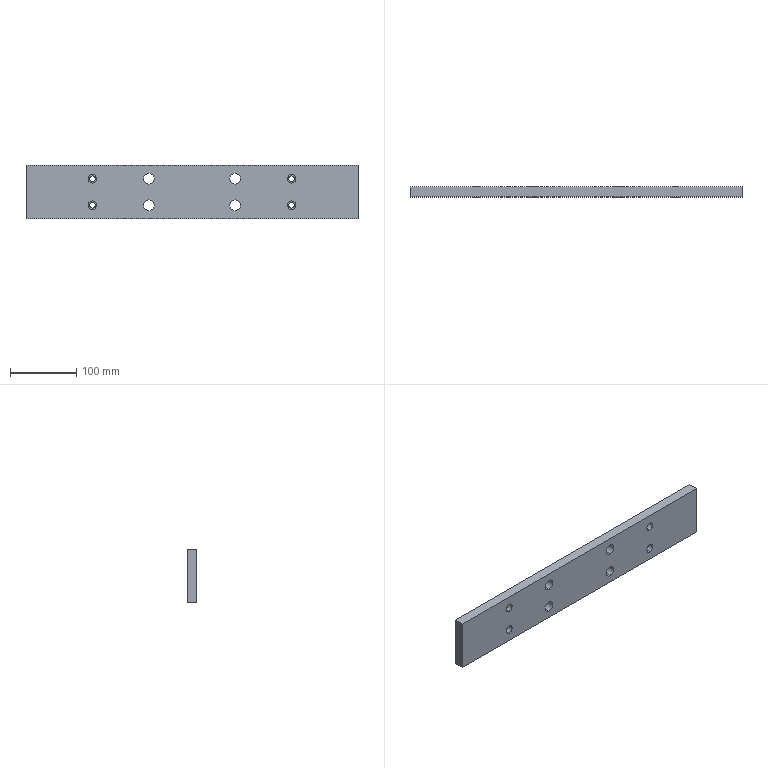Part | SolidWorks | features BaseBody 1 | 1 solid | 34 faces | box 500 x 15 x 80 mm | volume 581983 mm3 | cylinder 24 | plane 10 | commonest cylinder face diameters 8.4 x8 13 x8 16 x8
STEP:
#1=CARTESIAN_POINT('',(150.,92.,158.921));
#2=VERTEX_POINT('',#1);
#3=CARTESIAN_POINT('',(150.,92.,167.321));
#4=VERTEX_POINT('',#3);
#5=CARTESIAN_POINT('',(150.,92.,163.121));
#6=DIRECTION('',(0.,1.,0.));
#7=DIRECTION('',(0.,0.,-1.));
#8=AXIS2_PLACEMENT_3D('',#5,#6,#7);
#9=CIRCLE('',#8,4.2);
#10=EDGE_CURVE('',#2,#4,#9,.T.);
#11=ORIENTED_EDGE('',*,*,#10,.T.);
#12=CARTESIAN_POINT('',(150.,85.5,167.321));
#13=VERTEX_POINT('',#12);
#14=CARTESIAN_POINT('',(150.,77.,167.321));
#15=DIRECTION('',(0.,-1.,0.));
#16=VECTOR('',#15,1000.);
#17=LINE('',#14,#16);
#18=EDGE_CURVE('',#4,#13,#17,.T.);
#19=ORIENTED_EDGE('',*,*,#18,.T.);
#20=CARTESIAN_POINT('',(150.,85.5,158.921));
#21=VERTEX_POINT('',#20);
#22=CARTESIAN_POINT('',(150.,85.5,163.121));
#23=DIRECTION('',(0.,1.,0.));
#24=DIRECTION('',(0.,0.,-1.));
#25=AXIS2_PLACEMENT_3D('',#22,#23,#24);
#26=CIRCLE('',#25,4.2);
#27=EDGE_CURVE('',#21,#13,#26,.T.);
#28=ORIENTED_EDGE('',*,*,#27,.F.);
#29=CARTESIAN_POINT('',(150.,77.,158.921));
#30=DIRECTION('',(0.,-1.,0.));
#31=VECTOR('',#30,1000.);
#32=LINE('',#29,#31);
#33=EDGE_CURVE('',#2,#21,#32,.T.);
#34=ORIENTED_EDGE('',*,*,#33,.F.);
#35=EDGE_LOOP('',(#11,#19,#28,#34));
#36=FACE_OUTER_BOUND('',#35,.T.);
#37=CARTESIAN_POINT('',(150.,77.,163.121));
#38=DIRECTION('',(0.,-1.,0.));
#39=DIRECTION('',(0.,0.,-1.));
#40=AXIS2_PLACEMENT_3D('',#37,#38,#39);
#41=CYLINDRICAL_SURFACE('',#40,4.2);
#42=ADVANCED_FACE('',(#36),#41,.F.);
#43=CARTESIAN_POINT('',(150.,92.,118.921));
#44=VERTEX_POINT('',#43);
#45=CARTESIAN_POINT('',(150.,92.,127.321));
#46=VERTEX_POINT('',#45);
#47=CARTESIAN_POINT('',(150.,92.,123.121));
#48=DIRECTION('',(0.,1.,0.));
#49=DIRECTION('',(0.,0.,-1.));
#50=AXIS2_PLACEMENT_3D('',#47,#48,#49);
#51=CIRCLE('',#50,4.2);
#52=EDGE_CURVE('',#44,#46,#51,.T.);
#53=ORIENTED_EDGE('',*,*,#52,.T.);
#54=CARTESIAN_POINT('',(150.,85.5,127.321));
#55=VERTEX_POINT('',#54);
#56=CARTESIAN_POINT('',(150.,77.,127.321));
#57=DIRECTION('',(0.,-1.,0.));
#58=VECTOR('',#57,1000.);
#59=LINE('',#56,#58);
#60=EDGE_CURVE('',#46,#55,#59,.T.);
#61=ORIENTED_EDGE('',*,*,#60,.T.);
#62=CARTESIAN_POINT('',(150.,85.5,118.921));
#63=VERTEX_POINT('',#62);
#64=CARTESIAN_POINT('',(150.,85.5,123.121));
#65=DIRECTION('',(0.,1.,0.));
#66=DIRECTION('',(0.,0.,-1.));
#67=AXIS2_PLACEMENT_3D('',#64,#65,#66);
#68=CIRCLE('',#67,4.2);
#69=EDGE_CURVE('',#63,#55,#68,.T.);
#70=ORIENTED_EDGE('',*,*,#69,.F.);
#71=CARTESIAN_POINT('',(150.,77.,118.921));
#72=DIRECTION('',(0.,-1.,0.));
#73=VECTOR('',#72,1000.);
#74=LINE('',#71,#73);
#75=EDGE_CURVE('',#44,#63,#74,.T.);
#76=ORIENTED_EDGE('',*,*,#75,.F.);
#77=EDGE_LOOP('',(#53,#61,#70,#76));
#78=FACE_OUTER_BOUND('',#77,.T.);
#79=CARTESIAN_POINT('',(150.,77.,123.121));
#80=DIRECTION('',(0.,-1.,0.));
#81=DIRECTION('',(0.,0.,-1.));
#82=AXIS2_PLACEMENT_3D('',#79,#80,#81);
#83=CYLINDRICAL_SURFACE('',#82,4.2);
#84=ADVANCED_FACE('',(#78),#83,.F.);
#85=CARTESIAN_POINT('',(-150.,92.,158.921));
#86=VERTEX_POINT('',#85);
#87=CARTESIAN_POINT('',(-150.,92.,167.321));
#88=VERTEX_POINT('',#87);
#89=CARTESIAN_POINT('',(-150.,92.,163.121));
#90=DIRECTION('',(0.,1.,0.));
#91=DIRECTION('',(0.,0.,-1.));
#92=AXIS2_PLACEMENT_3D('',#89,#90,#91);
#93=CIRCLE('',#92,4.2);
#94=EDGE_CURVE('',#86,#88,#93,.T.);
#95=ORIENTED_EDGE('',*,*,#94,.T.);
#96=CARTESIAN_POINT('',(-150.,85.5,167.321));
#97=VERTEX_POINT('',#96);
#98=CARTESIAN_POINT('',(-150.,77.,167.321));
#99=DIRECTION('',(0.,-1.,0.));
#100=VECTOR('',#99,1000.);
#101=LINE('',#98,#100);
#102=EDGE_CURVE('',#88,#97,#101,.T.);
#103=ORIENTED_EDGE('',*,*,#102,.T.);
#104=CARTESIAN_POINT('',(-150.,85.5,158.921));
#105=VERTEX_POINT('',#104);
#106=CARTESIAN_POINT('',(-150.,85.5,163.121));
#107=DIRECTION('',(0.,1.,0.));
#108=DIRECTION('',(0.,0.,-1.));
#109=AXIS2_PLACEMENT_3D('',#106,#107,#108);
#110=CIRCLE('',#109,4.2);
#111=EDGE_CURVE('',#105,#97,#110,.T.);
#112=ORIENTED_EDGE('',*,*,#111,.F.);
#113=CARTESIAN_POINT('',(-150.,77.,158.921));
#114=DIRECTION('',(0.,-1.,0.));
#115=VECTOR('',#114,1000.);
#116=LINE('',#113,#115);
#117=EDGE_CURVE('',#86,#105,#116,.T.);
#118=ORIENTED_EDGE('',*,*,#117,.F.);
#119=EDGE_LOOP('',(#95,#103,#112,#118));
#120=FACE_OUTER_BOUND('',#119,.T.);
#121=CARTESIAN_POINT('',(-150.,77.,163.121));
#122=DIRECTION('',(0.,-1.,0.));
#123=DIRECTION('',(0.,0.,-1.));
#124=AXIS2_PLACEMENT_3D('',#121,#122,#123);
#125=CYLINDRICAL_SURFACE('',#124,4.2);
#126=ADVANCED_FACE('',(#120),#125,.F.);
#127=CARTESIAN_POINT('',(-150.,92.,118.921));
#128=VERTEX_POINT('',#127);
#129=CARTESIAN_POINT('',(-150.,92.,127.321));
#130=VERTEX_POINT('',#129);
#131=CARTESIAN_POINT('',(-150.,92.,123.121));
#132=DIRECTION('',(0.,1.,0.));
#133=DIRECTION('',(0.,0.,-1.));
#134=AXIS2_PLACEMENT_3D('',#131,#132,#133);
#135=CIRCLE('',#134,4.2);
#136=EDGE_CURVE('',#128,#130,#135,.T.);
#137=ORIENTED_EDGE('',*,*,#136,.T.);
#138=CARTESIAN_POINT('',(-150.,85.5,127.321));
#139=VERTEX_POINT('',#138);
#140=CARTESIAN_POINT('',(-150.,77.,127.321));
#141=DIRECTION('',(0.,-1.,0.));
#142=VECTOR('',#141,1000.);
#143=LINE('',#140,#142);
#144=EDGE_CURVE('',#130,#139,#143,.T.);
#145=ORIENTED_EDGE('',*,*,#144,.T.);
#146=CARTESIAN_POINT('',(-150.,85.5,118.921));
#147=VERTEX_POINT('',#146);
#148=CARTESIAN_POINT('',(-150.,85.5,123.121));
#149=DIRECTION('',(0.,1.,0.));
#150=DIRECTION('',(0.,0.,-1.));
#151=AXIS2_PLACEMENT_3D('',#148,#149,#150);
#152=CIRCLE('',#151,4.2);
#153=EDGE_CURVE('',#147,#139,#152,.T.);
#154=ORIENTED_EDGE('',*,*,#153,.F.);
#155=CARTESIAN_POINT('',(-150.,77.,118.921));
#156=DIRECTION('',(0.,-1.,0.));
#157=VECTOR('',#156,1000.);
#158=LINE('',#155,#157);
#159=EDGE_CURVE('',#128,#147,#158,.T.);
#160=ORIENTED_EDGE('',*,*,#159,.F.);
#161=EDGE_LOOP('',(#137,#145,#154,#160));
#162=FACE_OUTER_BOUND('',#161,.T.);
#163=CARTESIAN_POINT('',(-150.,77.,123.121));
#164=DIRECTION('',(0.,-1.,0.));
#165=DIRECTION('',(0.,0.,-1.));
#166=AXIS2_PLACEMENT_3D('',#163,#164,#165);
#167=CYLINDRICAL_SURFACE('',#166,4.2);
#168=ADVANCED_FACE('',(#162),#167,.F.);
#169=CARTESIAN_POINT('',(65.,92.,115.121));
#170=VERTEX_POINT('',#169);
#171=CARTESIAN_POINT('',(65.,92.,131.121));
#172=VERTEX_POINT('',#171);
#173=CARTESIAN_POINT('',(65.,92.,123.121));
#174=DIRECTION('',(0.,1.,0.));
#175=DIRECTION('',(0.,0.,-1.));
#176=AXIS2_PLACEMENT_3D('',#173,#174,#175);
#177=CIRCLE('',#176,8.);
#178=EDGE_CURVE('',#170,#172,#177,.T.);
#179=ORIENTED_EDGE('',*,*,#178,.T.);
#180=CARTESIAN_POINT('',(65.,77.,131.121));
#181=VERTEX_POINT('',#180);
#182=CARTESIAN_POINT('',(65.,77.,131.121));
#183=DIRECTION('',(0.,-1.,0.));
#184=VECTOR('',#183,1000.);
#185=LINE('',#182,#184);
#186=EDGE_CURVE('',#172,#181,#185,.T.);
#187=ORIENTED_EDGE('',*,*,#186,.T.);
#188=CARTESIAN_POINT('',(65.,77.,115.121));
#189=VERTEX_POINT('',#188);
#190=CARTESIAN_POINT('',(65.,77.,123.121));
#191=DIRECTION('',(0.,1.,0.));
#192=DIRECTION('',(0.,0.,-1.));
#193=AXIS2_PLACEMENT_3D('',#190,#191,#192);
#194=CIRCLE('',#193,8.);
#195=EDGE_CURVE('',#189,#181,#194,.T.);
#196=ORIENTED_EDGE('',*,*,#195,.F.);
#197=CARTESIAN_POINT('',(65.,77.,115.121));
#198=DIRECTION('',(0.,-1.,0.));
#199=VECTOR('',#198,1000.);
#200=LINE('',#197,#199);
#201=EDGE_CURVE('',#170,#189,#200,.T.);
#202=ORIENTED_EDGE('',*,*,#201,.F.);
#203=EDGE_LOOP('',(#179,#187,#196,#202));
#204=FACE_OUTER_BOUND('',#203,.T.);
#205=CARTESIAN_POINT('',(65.,77.,123.121));
#206=DIRECTION('',(0.,-1.,0.));
#207=DIRECTION('',(0.,0.,-1.));
#208=AXIS2_PLACEMENT_3D('',#205,#206,#207);
#209=CYLINDRICAL_SURFACE('',#208,8.);
#210=ADVANCED_FACE('',(#204),#209,.F.);
#211=CARTESIAN_POINT('',(65.,92.,155.121));
#212=VERTEX_POINT('',#211);
#213=CARTESIAN_POINT('',(65.,92.,171.121));
#214=VERTEX_POINT('',#213);
#215=CARTESIAN_POINT('',(65.,92.,163.121));
#216=DIRECTION('',(0.,1.,0.));
#217=DIRECTION('',(0.,0.,-1.));
#218=AXIS2_PLACEMENT_3D('',#215,#216,#217);
#219=CIRCLE('',#218,8.);
#220=EDGE_CURVE('',#212,#214,#219,.T.);
#221=ORIENTED_EDGE('',*,*,#220,.T.);
#222=CARTESIAN_POINT('',(65.,77.,171.121));
#223=VERTEX_POINT('',#222);
#224=CARTESIAN_POINT('',(65.,77.,171.121));
#225=DIRECTION('',(0.,-1.,0.));
#226=VECTOR('',#225,1000.);
#227=LINE('',#224,#226);
#228=EDGE_CURVE('',#214,#223,#227,.T.);
#229=ORIENTED_EDGE('',*,*,#228,.T.);
#230=CARTESIAN_POINT('',(65.,77.,155.121));
#231=VERTEX_POINT('',#230);
#232=CARTESIAN_POINT('',(65.,77.,163.121));
#233=DIRECTION('',(0.,1.,0.));
#234=DIRECTION('',(0.,0.,-1.));
#235=AXIS2_PLACEMENT_3D('',#232,#233,#234);
#236=CIRCLE('',#235,8.);
#237=EDGE_CURVE('',#231,#223,#236,.T.);
#238=ORIENTED_EDGE('',*,*,#237,.F.);
#239=CARTESIAN_POINT('',(65.,77.,155.121));
#240=DIRECTION('',(0.,-1.,0.));
#241=VECTOR('',#240,1000.);
#242=LINE('',#239,#241);
#243=EDGE_CURVE('',#212,#231,#242,.T.);
#244=ORIENTED_EDGE('',*,*,#243,.F.);
#245=EDGE_LOOP('',(#221,#229,#238,#244));
#246=FACE_OUTER_BOUND('',#245,.T.);
#247=CARTESIAN_POINT('',(65.,77.,163.121));
#248=DIRECTION('',(0.,-1.,0.));
#249=DIRECTION('',(0.,0.,-1.));
#250=AXIS2_PLACEMENT_3D('',#247,#248,#249);
#251=CYLINDRICAL_SURFACE('',#250,8.);
#252=ADVANCED_FACE('',(#246),#251,.F.);
#253=CARTESIAN_POINT('',(-65.,92.,115.121));
#254=VERTEX_POINT('',#253);
#255=CARTESIAN_POINT('',(-65.,92.,131.121));
#256=VERTEX_POINT('',#255);
#257=CARTESIAN_POINT('',(-65.,92.,123.121));
#258=DIRECTION('',(0.,1.,0.));
#259=DIRECTION('',(0.,0.,-1.));
#260=AXIS2_PLACEMENT_3D('',#257,#258,#259);
#261=CIRCLE('',#260,8.);
#262=EDGE_CURVE('',#254,#256,#261,.T.);
#263=ORIENTED_EDGE('',*,*,#262,.T.);
#264=CARTESIAN_POINT('',(-65.,77.,131.121));
#265=VERTEX_POINT('',#264);
#266=CARTESIAN_POINT('',(-65.,77.,131.121));
#267=DIRECTION('',(0.,-1.,0.));
#268=VECTOR('',#267,1000.);
#269=LINE('',#266,#268);
#270=EDGE_CURVE('',#256,#265,#269,.T.);
#271=ORIENTED_EDGE('',*,*,#270,.T.);
#272=CARTESIAN_POINT('',(-65.,77.,115.121));
#273=VERTEX_POINT('',#272);
#274=CARTESIAN_POINT('',(-65.,77.,123.121));
#275=DIRECTION('',(0.,1.,0.));
#276=DIRECTION('',(0.,0.,-1.));
#277=AXIS2_PLACEMENT_3D('',#274,#275,#276);
#278=CIRCLE('',#277,8.);
#279=EDGE_CURVE('',#273,#265,#278,.T.);
#280=ORIENTED_EDGE('',*,*,#279,.F.);
#281=CARTESIAN_POINT('',(-65.,77.,115.121));
#282=DIRECTION('',(0.,-1.,0.));
#283=VECTOR('',#282,1000.);
#284=LINE('',#281,#283);
#285=EDGE_CURVE('',#254,#273,#284,.T.);
#286=ORIENTED_EDGE('',*,*,#285,.F.);
#287=EDGE_LOOP('',(#263,#271,#280,#286));
#288=FACE_OUTER_BOUND('',#287,.T.);
#289=CARTESIAN_POINT('',(-65.,77.,123.121));
#290=DIRECTION('',(0.,-1.,0.));
#291=DIRECTION('',(0.,0.,-1.));
#292=AXIS2_PLACEMENT_3D('',#289,#290,#291);
#293=CYLINDRICAL_SURFACE('',#292,8.);
#294=ADVANCED_FACE('',(#288),#293,.F.);
#295=CARTESIAN_POINT('',(-65.,92.,155.121));
#296=VERTEX_POINT('',#295);
#297=CARTESIAN_POINT('',(-65.,92.,171.121));
#298=VERTEX_POINT('',#297);
#299=CARTESIAN_POINT('',(-65.,92.,163.121));
#300=DIRECTION('',(0.,1.,0.));
#301=DIRECTION('',(0.,0.,-1.));
#302=AXIS2_PLACEMENT_3D('',#299,#300,#301);
#303=CIRCLE('',#302,8.);
#304=EDGE_CURVE('',#296,#298,#303,.T.);
#305=ORIENTED_EDGE('',*,*,#304,.T.);
#306=CARTESIAN_POINT('',(-65.,77.,171.121));
#307=VERTEX_POINT('',#306);
#308=CARTESIAN_POINT('',(-65.,77.,171.121));
#309=DIRECTION('',(0.,-1.,0.));
#310=VECTOR('',#309,1000.);
#311=LINE('',#308,#310);
#312=EDGE_CURVE('',#298,#307,#311,.T.);
#313=ORIENTED_EDGE('',*,*,#312,.T.);
#314=CARTESIAN_POINT('',(-65.,77.,155.121));
#315=VERTEX_POINT('',#314);
#316=CARTESIAN_POINT('',(-65.,77.,163.121));
#317=DIRECTION('',(0.,1.,0.));
#318=DIRECTION('',(0.,0.,-1.));
#319=AXIS2_PLACEMENT_3D('',#316,#317,#318);
#320=CIRCLE('',#319,8.);
#321=EDGE_CURVE('',#315,#307,#320,.T.);
#322=ORIENTED_EDGE('',*,*,#321,.F.);
#323=CARTESIAN_POINT('',(-65.,77.,155.121));
#324=DIRECTION('',(0.,-1.,0.));
#325=VECTOR('',#324,1000.);
#326=LINE('',#323,#325);
#327=EDGE_CURVE('',#296,#315,#326,.T.);
#328=ORIENTED_EDGE('',*,*,#327,.F.);
#329=EDGE_LOOP('',(#305,#313,#322,#328));
#330=FACE_OUTER_BOUND('',#329,.T.);
#331=CARTESIAN_POINT('',(-65.,77.,163.121));
#332=DIRECTION('',(0.,-1.,0.));
#333=DIRECTION('',(0.,0.,-1.));
#334=AXIS2_PLACEMENT_3D('',#331,#332,#333);
#335=CYLINDRICAL_SURFACE('',#334,8.);
#336=ADVANCED_FACE('',(#330),#335,.F.);
#337=CARTESIAN_POINT('',(150.,85.5,156.621));
#338=VERTEX_POINT('',#337);
#339=CARTESIAN_POINT('',(150.,85.5,169.621));
#340=VERTEX_POINT('',#339);
#341=CARTESIAN_POINT('',(150.,85.5,163.121));
#342=DIRECTION('',(0.,1.,0.));
#343=DIRECTION('',(0.,0.,-1.));
#344=AXIS2_PLACEMENT_3D('',#341,#342,#343);
#345=CIRCLE('',#344,6.5);
#346=EDGE_CURVE('',#338,#340,#345,.T.);
#347=ORIENTED_EDGE('',*,*,#346,.T.);
#348=CARTESIAN_POINT('',(150.,77.,169.621));
#349=VERTEX_POINT('',#348);
#350=CARTESIAN_POINT('',(150.,77.,169.621));
#351=DIRECTION('',(0.,-1.,0.));
#352=VECTOR('',#351,1000.);
#353=LINE('',#350,#352);
#354=EDGE_CURVE('',#340,#349,#353,.T.);
#355=ORIENTED_EDGE('',*,*,#354,.T.);
#356=CARTESIAN_POINT('',(150.,77.,156.621));
#357=VERTEX_POINT('',#356);
#358=CARTESIAN_POINT('',(150.,77.,163.121));
#359=DIRECTION('',(0.,1.,0.));
#360=DIRECTION('',(0.,0.,-1.));
#361=AXIS2_PLACEMENT_3D('',#358,#359,#360);
#362=CIRCLE('',#361,6.5);
#363=EDGE_CURVE('',#357,#349,#362,.T.);
#364=ORIENTED_EDGE('',*,*,#363,.F.);
#365=CARTESIAN_POINT('',(150.,77.,156.621));
#366=DIRECTION('',(0.,-1.,0.));
#367=VECTOR('',#366,1000.);
#368=LINE('',#365,#367);
#369=EDGE_CURVE('',#338,#357,#368,.T.);
#370=ORIENTED_EDGE('',*,*,#369,.F.);
#371=EDGE_LOOP('',(#347,#355,#364,#370));
#372=FACE_OUTER_BOUND('',#371,.T.);
#373=CARTESIAN_POINT('',(150.,77.,163.121));
#374=DIRECTION('',(0.,-1.,0.));
#375=DIRECTION('',(0.,0.,-1.));
#376=AXIS2_PLACEMENT_3D('',#373,#374,#375);
#377=CYLINDRICAL_SURFACE('',#376,6.5);
#378=ADVANCED_FACE('',(#372),#377,.F.);
#379=CARTESIAN_POINT('',(150.,85.5,116.621));
#380=VERTEX_POINT('',#379);
#381=CARTESIAN_POINT('',(150.,85.5,129.621));
#382=VERTEX_POINT('',#381);
#383=CARTESIAN_POINT('',(150.,85.5,123.121));
#384=DIRECTION('',(0.,1.,0.));
#385=DIRECTION('',(0.,0.,-1.));
#386=AXIS2_PLACEMENT_3D('',#383,#384,#385);
#387=CIRCLE('',#386,6.5);
#388=EDGE_CURVE('',#380,#382,#387,.T.);
#389=ORIENTED_EDGE('',*,*,#388,.T.);
#390=CARTESIAN_POINT('',(150.,77.,129.621));
#391=VERTEX_POINT('',#390);
#392=CARTESIAN_POINT('',(150.,77.,129.621));
#393=DIRECTION('',(0.,-1.,0.));
#394=VECTOR('',#393,1000.);
#395=LINE('',#392,#394);
#396=EDGE_CURVE('',#382,#391,#395,.T.);
#397=ORIENTED_EDGE('',*,*,#396,.T.);
#398=CARTESIAN_POINT('',(150.,77.,116.621));
#399=VERTEX_POINT('',#398);
#400=CARTESIAN_POINT('',(150.,77.,123.121));
#401=DIRECTION('',(0.,1.,0.));
#402=DIRECTION('',(0.,0.,-1.));
#403=AXIS2_PLACEMENT_3D('',#400,#401,#402);
#404=CIRCLE('',#403,6.5);
#405=EDGE_CURVE('',#399,#391,#404,.T.);
#406=ORIENTED_EDGE('',*,*,#405,.F.);
#407=CARTESIAN_POINT('',(150.,77.,116.621));
#408=DIRECTION('',(0.,-1.,0.));
#409=VECTOR('',#408,1000.);
#410=LINE('',#407,#409);
#411=EDGE_CURVE('',#380,#399,#410,.T.);
#412=ORIENTED_EDGE('',*,*,#411,.F.);
#413=EDGE_LOOP('',(#389,#397,#406,#412));
#414=FACE_OUTER_BOUND('',#413,.T.);
#415=CARTESIAN_POINT('',(150.,77.,123.121));
#416=DIRECTION('',(0.,-1.,0.));
#417=DIRECTION('',(0.,0.,-1.));
#418=AXIS2_PLACEMENT_3D('',#415,#416,#417);
#419=CYLINDRICAL_SURFACE('',#418,6.5);
#420=ADVANCED_FACE('',(#414),#419,.F.);
#421=CARTESIAN_POINT('',(-150.,85.5,156.621));
#422=VERTEX_POINT('',#421);
#423=CARTESIAN_POINT('',(-150.,85.5,169.621));
#424=VERTEX_POINT('',#423);
#425=CARTESIAN_POINT('',(-150.,85.5,163.121));
#426=DIRECTION('',(0.,1.,0.));
#427=DIRECTION('',(0.,0.,-1.));
#428=AXIS2_PLACEMENT_3D('',#425,#426,#427);
#429=CIRCLE('',#428,6.5);
#430=EDGE_CURVE('',#422,#424,#429,.T.);
#431=ORIENTED_EDGE('',*,*,#430,.T.);
#432=CARTESIAN_POINT('',(-150.,77.,169.621));
#433=VERTEX_POINT('',#432);
#434=CARTESIAN_POINT('',(-150.,77.,169.621));
#435=DIRECTION('',(0.,-1.,0.));
#436=VECTOR('',#435,1000.);
#437=LINE('',#434,#436);
#438=EDGE_CURVE('',#424,#433,#437,.T.);
#439=ORIENTED_EDGE('',*,*,#438,.T.);
#440=CARTESIAN_POINT('',(-150.,77.,156.621));
#441=VERTEX_POINT('',#440);
#442=CARTESIAN_POINT('',(-150.,77.,163.121));
#443=DIRECTION('',(0.,1.,0.));
#444=DIRECTION('',(0.,0.,-1.));
#445=AXIS2_PLACEMENT_3D('',#442,#443,#444);
#446=CIRCLE('',#445,6.5);
#447=EDGE_CURVE('',#441,#433,#446,.T.);
#448=ORIENTED_EDGE('',*,*,#447,.F.);
#449=CARTESIAN_POINT('',(-150.,77.,156.621));
#450=DIRECTION('',(0.,-1.,0.));
#451=VECTOR('',#450,1000.);
#452=LINE('',#449,#451);
#453=EDGE_CURVE('',#422,#441,#452,.T.);
#454=ORIENTED_EDGE('',*,*,#453,.F.);
#455=EDGE_LOOP('',(#431,#439,#448,#454));
#456=FACE_OUTER_BOUND('',#455,.T.);
#457=CARTESIAN_POINT('',(-150.,77.,163.121));
#458=DIRECTION('',(0.,-1.,0.));
#459=DIRECTION('',(0.,0.,-1.));
#460=AXIS2_PLACEMENT_3D('',#457,#458,#459);
#461=CYLINDRICAL_SURFACE('',#460,6.5);
#462=ADVANCED_FACE('',(#456),#461,.F.);
#463=CARTESIAN_POINT('',(-150.,85.5,116.621));
#464=VERTEX_POINT('',#463);
#465=CARTESIAN_POINT('',(-150.,85.5,129.621));
#466=VERTEX_POINT('',#465);
#467=CARTESIAN_POINT('',(-150.,85.5,123.121));
#468=DIRECTION('',(0.,1.,0.));
#469=DIRECTION('',(0.,0.,-1.));
#470=AXIS2_PLACEMENT_3D('',#467,#468,#469);
#471=CIRCLE('',#470,6.5);
#472=EDGE_CURVE('',#464,#466,#471,.T.);
#473=ORIENTED_EDGE('',*,*,#472,.T.);
#474=CARTESIAN_POINT('',(-150.,77.,129.621));
#475=VERTEX_POINT('',#474);
#476=CARTESIAN_POINT('',(-150.,77.,129.621));
#477=DIRECTION('',(0.,-1.,0.));
#478=VECTOR('',#477,1000.);
#479=LINE('',#476,#478);
#480=EDGE_CURVE('',#466,#475,#479,.T.);
#481=ORIENTED_EDGE('',*,*,#480,.T.);
#482=CARTESIAN_POINT('',(-150.,77.,116.621));
#483=VERTEX_POINT('',#482);
#484=CARTESIAN_POINT('',(-150.,77.,123.121));
#485=DIRECTION('',(0.,1.,0.));
#486=DIRECTION('',(0.,0.,-1.));
#487=AXIS2_PLACEMENT_3D('',#484,#485,#486);
#488=CIRCLE('',#487,6.5);
#489=EDGE_CURVE('',#483,#475,#488,.T.);
#490=ORIENTED_EDGE('',*,*,#489,.F.);
#491=CARTESIAN_POINT('',(-150.,77.,116.621));
#492=DIRECTION('',(0.,-1.,0.));
#493=VECTOR('',#492,1000.);
#494=LINE('',#491,#493);
#495=EDGE_CURVE('',#464,#483,#494,.T.);
#496=ORIENTED_EDGE('',*,*,#495,.F.);
#497=EDGE_LOOP('',(#473,#481,#490,#496));
#498=FACE_OUTER_BOUND('',#497,.T.);
#499=CARTESIAN_POINT('',(-150.,77.,123.121));
#500=DIRECTION('',(0.,-1.,0.));
#501=DIRECTION('',(0.,0.,-1.));
#502=AXIS2_PLACEMENT_3D('',#499,#500,#501);
#503=CYLINDRICAL_SURFACE('',#502,6.5);
#504=ADVANCED_FACE('',(#498),#503,.F.);
#505=CARTESIAN_POINT('',(250.,92.,183.121));
#506=VERTEX_POINT('',#505);
#507=CARTESIAN_POINT('',(-250.,92.,183.121));
#508=VERTEX_POINT('',#507);
#509=CARTESIAN_POINT('',(0.,92.,183.121));
#510=DIRECTION('',(-1.,0.,0.));
#511=VECTOR('',#510,1000.);
#512=LINE('',#509,#511);
#513=EDGE_CURVE('',#506,#508,#512,.T.);
#514=ORIENTED_EDGE('',*,*,#513,.F.);
#515=CARTESIAN_POINT('',(250.,92.,103.121));
#516=VERTEX_POINT('',#515);
#517=CARTESIAN_POINT('',(250.,92.,143.121));
#518=DIRECTION('',(0.,0.,1.));
#519=VECTOR('',#518,1000.);
#520=LINE('',#517,#519);
#521=EDGE_CURVE('',#516,#506,#520,.T.);
#522=ORIENTED_EDGE('',*,*,#521,.F.);
#523=CARTESIAN_POINT('',(-250.,92.,103.121));
#524=VERTEX_POINT('',#523);
#525=CARTESIAN_POINT('',(0.,92.,103.121));
#526=DIRECTION('',(1.,0.,0.));
#527=VECTOR('',#526,1000.);
#528=LINE('',#525,#527);
#529=EDGE_CURVE('',#524,#516,#528,.T.);
#530=ORIENTED_EDGE('',*,*,#529,.F.);
#531=CARTESIAN_POINT('',(-250.,92.,143.121));
#532=DIRECTION('',(0.,0.,-1.));
#533=VECTOR('',#532,1000.);
#534=LINE('',#531,#533);
#535=EDGE_CURVE('',#508,#524,#534,.T.);
#536=ORIENTED_EDGE('',*,*,#535,.F.);
#537=EDGE_LOOP('',(#514,#522,#530,#536));
#538=FACE_OUTER_BOUND('',#537,.T.);
#539=ORIENTED_EDGE('',*,*,#10,.F.);
#540=CARTESIAN_POINT('',(150.,92.,163.121));
#541=DIRECTION('',(0.,1.,0.));
#542=DIRECTION('',(0.,0.,-1.));
#543=AXIS2_PLACEMENT_3D('',#540,#541,#542);
#544=CIRCLE('',#543,4.2);
#545=EDGE_CURVE('',#4,#2,#544,.T.);
#546=ORIENTED_EDGE('',*,*,#545,.F.);
#547=EDGE_LOOP('',(#539,#546));
#548=FACE_BOUND('',#547,.T.);
#549=ORIENTED_EDGE('',*,*,#52,.F.);
#550=CARTESIAN_POINT('',(150.,92.,123.121));
#551=DIRECTION('',(0.,1.,0.));
#552=DIRECTION('',(0.,0.,-1.));
#553=AXIS2_PLACEMENT_3D('',#550,#551,#552);
#554=CIRCLE('',#553,4.2);
#555=EDGE_CURVE('',#46,#44,#554,.T.);
#556=ORIENTED_EDGE('',*,*,#555,.F.);
#557=EDGE_LOOP('',(#549,#556));
#558=FACE_BOUND('',#557,.T.);
#559=ORIENTED_EDGE('',*,*,#94,.F.);
#560=CARTESIAN_POINT('',(-150.,92.,163.121));
#561=DIRECTION('',(0.,1.,0.));
#562=DIRECTION('',(0.,0.,-1.));
#563=AXIS2_PLACEMENT_3D('',#560,#561,#562);
#564=CIRCLE('',#563,4.2);
#565=EDGE_CURVE('',#88,#86,#564,.T.);
#566=ORIENTED_EDGE('',*,*,#565,.F.);
#567=EDGE_LOOP('',(#559,#566));
#568=FACE_BOUND('',#567,.T.);
#569=ORIENTED_EDGE('',*,*,#136,.F.);
#570=CARTESIAN_POINT('',(-150.,92.,123.121));
#571=DIRECTION('',(0.,1.,0.));
#572=DIRECTION('',(0.,0.,-1.));
#573=AXIS2_PLACEMENT_3D('',#570,#571,#572);
#574=CIRCLE('',#573,4.2);
#575=EDGE_CURVE('',#130,#128,#574,.T.);
#576=ORIENTED_EDGE('',*,*,#575,.F.);
#577=EDGE_LOOP('',(#569,#576));
#578=FACE_BOUND('',#577,.T.);
#579=ORIENTED_EDGE('',*,*,#178,.F.);
#580=CARTESIAN_POINT('',(65.,92.,123.121));
#581=DIRECTION('',(0.,1.,0.));
#582=DIRECTION('',(0.,0.,-1.));
#583=AXIS2_PLACEMENT_3D('',#580,#581,#582);
#584=CIRCLE('',#583,8.);
#585=EDGE_CURVE('',#172,#170,#584,.T.);
#586=ORIENTED_EDGE('',*,*,#585,.F.);
#587=EDGE_LOOP('',(#579,#586));
#588=FACE_BOUND('',#587,.T.);
#589=ORIENTED_EDGE('',*,*,#220,.F.);
#590=CARTESIAN_POINT('',(65.,92.,163.121));
#591=DIRECTION('',(0.,1.,0.));
#592=DIRECTION('',(0.,0.,-1.));
#593=AXIS2_PLACEMENT_3D('',#590,#591,#592);
#594=CIRCLE('',#593,8.);
#595=EDGE_CURVE('',#214,#212,#594,.T.);
#596=ORIENTED_EDGE('',*,*,#595,.F.);
#597=EDGE_LOOP('',(#589,#596));
#598=FACE_BOUND('',#597,.T.);
#599=ORIENTED_EDGE('',*,*,#262,.F.);
#600=CARTESIAN_POINT('',(-65.,92.,123.121));
#601=DIRECTION('',(0.,1.,0.));
#602=DIRECTION('',(0.,0.,-1.));
#603=AXIS2_PLACEMENT_3D('',#600,#601,#602);
#604=CIRCLE('',#603,8.);
#605=EDGE_CURVE('',#256,#254,#604,.T.);
#606=ORIENTED_EDGE('',*,*,#605,.F.);
#607=EDGE_LOOP('',(#599,#606));
#608=FACE_BOUND('',#607,.T.);
#609=ORIENTED_EDGE('',*,*,#304,.F.);
#610=CARTESIAN_POINT('',(-65.,92.,163.121));
#611=DIRECTION('',(0.,1.,0.));
#612=DIRECTION('',(0.,0.,-1.));
#613=AXIS2_PLACEMENT_3D('',#610,#611,#612);
#614=CIRCLE('',#613,8.);
#615=EDGE_CURVE('',#298,#296,#614,.T.);
#616=ORIENTED_EDGE('',*,*,#615,.F.);
#617=EDGE_LOOP('',(#609,#616));
#618=FACE_BOUND('',#617,.T.);
#619=CARTESIAN_POINT('',(0.,92.,143.121));
#620=DIRECTION('',(0.,-1.,0.));
#621=DIRECTION('',(0.,0.,-1.));
#622=AXIS2_PLACEMENT_3D('',#619,#620,#621);
#623=PLANE('',#622);
#624=ADVANCED_FACE('',(#538,#548,#558,#568,#578,#588,#598,#608,#618),#623,.F.);
#625=CARTESIAN_POINT('',(-250.,77.,103.121));
#626=VERTEX_POINT('',#625);
#627=CARTESIAN_POINT('',(-250.,77.,103.121));
#628=DIRECTION('',(0.,1.,0.));
#629=VECTOR('',#628,1000.);
#630=LINE('',#627,#629);
#631=EDGE_CURVE('',#626,#524,#630,.T.);
#632=ORIENTED_EDGE('',*,*,#631,.F.);
#633=CARTESIAN_POINT('',(-250.,77.,183.121));
#634=VERTEX_POINT('',#633);
#635=CARTESIAN_POINT('',(-250.,77.,103.121));
#636=DIRECTION('',(0.,0.,-1.));
#637=VECTOR('',#636,1000.);
#638=LINE('',#635,#637);
#639=EDGE_CURVE('',#634,#626,#638,.T.);
#640=ORIENTED_EDGE('',*,*,#639,.F.);
#641=CARTESIAN_POINT('',(-250.,77.,183.121));
#642=DIRECTION('',(0.,-1.,0.));
#643=VECTOR('',#642,1000.);
#644=LINE('',#641,#643);
#645=EDGE_CURVE('',#508,#634,#644,.T.);
#646=ORIENTED_EDGE('',*,*,#645,.F.);
#647=ORIENTED_EDGE('',*,*,#535,.T.);
#648=EDGE_LOOP('',(#632,#640,#646,#647));
#649=FACE_OUTER_BOUND('',#648,.T.);
#650=CARTESIAN_POINT('',(-250.,77.,103.121));
#651=DIRECTION('',(1.,0.,0.));
#652=DIRECTION('',(0.,0.,-1.));
#653=AXIS2_PLACEMENT_3D('',#650,#651,#652);
#654=PLANE('',#653);
#655=ADVANCED_FACE('',(#649),#654,.F.);
#656=ORIENTED_EDGE('',*,*,#645,.T.);
#657=CARTESIAN_POINT('',(250.,77.,183.121));
#658=VERTEX_POINT('',#657);
#659=CARTESIAN_POINT('',(250.,77.,183.121));
#660=DIRECTION('',(-1.,0.,0.));
#661=VECTOR('',#660,1000.);
#662=LINE('',#659,#661);
#663=EDGE_CURVE('',#658,#634,#662,.T.);
#664=ORIENTED_EDGE('',*,*,#663,.F.);
#665=CARTESIAN_POINT('',(250.,77.,183.121));
#666=DIRECTION('',(0.,-1.,0.));
#667=VECTOR('',#666,1000.);
#668=LINE('',#665,#667);
#669=EDGE_CURVE('',#506,#658,#668,.T.);
#670=ORIENTED_EDGE('',*,*,#669,.F.);
#671=ORIENTED_EDGE('',*,*,#513,.T.);
#672=EDGE_LOOP('',(#656,#664,#670,#671));
#673=FACE_OUTER_BOUND('',#672,.T.);
#674=CARTESIAN_POINT('',(250.,77.,183.121));
#675=DIRECTION('',(0.,0.,-1.));
#676=DIRECTION('',(-1.,0.,0.));
#677=AXIS2_PLACEMENT_3D('',#674,#675,#676);
#678=PLANE('',#677);
#679=ADVANCED_FACE('',(#673),#678,.F.);
#680=ORIENTED_EDGE('',*,*,#669,.T.);
#681=CARTESIAN_POINT('',(250.,77.,103.121));
#682=VERTEX_POINT('',#681);
#683=CARTESIAN_POINT('',(250.,77.,103.121));
#684=DIRECTION('',(0.,0.,1.));
#685=VECTOR('',#684,1000.);
#686=LINE('',#683,#685);
#687=EDGE_CURVE('',#682,#658,#686,.T.);
#688=ORIENTED_EDGE('',*,*,#687,.F.);
#689=CARTESIAN_POINT('',(250.,77.,103.121));
#690=DIRECTION('',(0.,-1.,0.));
#691=VECTOR('',#690,1000.);
#692=LINE('',#689,#691);
#693=EDGE_CURVE('',#516,#682,#692,.T.);
#694=ORIENTED_EDGE('',*,*,#693,.F.);
#695=ORIENTED_EDGE('',*,*,#521,.T.);
#696=EDGE_LOOP('',(#680,#688,#694,#695));
#697=FACE_OUTER_BOUND('',#696,.T.);
#698=CARTESIAN_POINT('',(250.,77.,103.121));
#699=DIRECTION('',(-1.,0.,0.));
#700=DIRECTION('',(0.,0.,1.));
#701=AXIS2_PLACEMENT_3D('',#698,#699,#700);
#702=PLANE('',#701);
#703=ADVANCED_FACE('',(#697),#702,.F.);
#704=ORIENTED_EDGE('',*,*,#693,.T.);
#705=CARTESIAN_POINT('',(250.,77.,103.121));
#706=DIRECTION('',(1.,0.,0.));
#707=VECTOR('',#706,1000.);
#708=LINE('',#705,#707);
#709=EDGE_CURVE('',#626,#682,#708,.T.);
#710=ORIENTED_EDGE('',*,*,#709,.F.);
#711=ORIENTED_EDGE('',*,*,#631,.T.);
#712=ORIENTED_EDGE('',*,*,#529,.T.);
#713=EDGE_LOOP('',(#704,#710,#711,#712));
#714=FACE_OUTER_BOUND('',#713,.T.);
#715=CARTESIAN_POINT('',(250.,77.,103.121));
#716=DIRECTION('',(0.,0.,1.));
#717=DIRECTION('',(1.,0.,0.));
#718=AXIS2_PLACEMENT_3D('',#715,#716,#717);
#719=PLANE('',#718);
#720=ADVANCED_FACE('',(#714),#719,.F.);
#721=ORIENTED_EDGE('',*,*,#18,.F.);
#722=ORIENTED_EDGE('',*,*,#545,.T.);
#723=ORIENTED_EDGE('',*,*,#33,.T.);
#724=CARTESIAN_POINT('',(150.,85.5,163.121));
#725=DIRECTION('',(0.,1.,0.));
#726=DIRECTION('',(0.,0.,-1.));
#727=AXIS2_PLACEMENT_3D('',#724,#725,#726);
#728=CIRCLE('',#727,4.2);
#729=EDGE_CURVE('',#13,#21,#728,.T.);
#730=ORIENTED_EDGE('',*,*,#729,.F.);
#731=EDGE_LOOP('',(#721,#722,#723,#730));
#732=FACE_OUTER_BOUND('',#731,.T.);
#733=CARTESIAN_POINT('',(150.,77.,163.121));
#734=DIRECTION('',(0.,-1.,0.));
#735=DIRECTION('',(0.,0.,-1.));
#736=AXIS2_PLACEMENT_3D('',#733,#734,#735);
#737=CYLINDRICAL_SURFACE('',#736,4.2);
#738=ADVANCED_FACE('',(#732),#737,.F.);
#739=ORIENTED_EDGE('',*,*,#60,.F.);
#740=ORIENTED_EDGE('',*,*,#555,.T.);
#741=ORIENTED_EDGE('',*,*,#75,.T.);
#742=CARTESIAN_POINT('',(150.,85.5,123.121));
#743=DIRECTION('',(0.,1.,0.));
#744=DIRECTION('',(0.,0.,-1.));
#745=AXIS2_PLACEMENT_3D('',#742,#743,#744);
#746=CIRCLE('',#745,4.2);
#747=EDGE_CURVE('',#55,#63,#746,.T.);
#748=ORIENTED_EDGE('',*,*,#747,.F.);
#749=EDGE_LOOP('',(#739,#740,#741,#748));
#750=FACE_OUTER_BOUND('',#749,.T.);
#751=CARTESIAN_POINT('',(150.,77.,123.121));
#752=DIRECTION('',(0.,-1.,0.));
#753=DIRECTION('',(0.,0.,-1.));
#754=AXIS2_PLACEMENT_3D('',#751,#752,#753);
#755=CYLINDRICAL_SURFACE('',#754,4.2);
#756=ADVANCED_FACE('',(#750),#755,.F.);
#757=ORIENTED_EDGE('',*,*,#102,.F.);
#758=ORIENTED_EDGE('',*,*,#565,.T.);
#759=ORIENTED_EDGE('',*,*,#117,.T.);
#760=CARTESIAN_POINT('',(-150.,85.5,163.121));
#761=DIRECTION('',(0.,1.,0.));
#762=DIRECTION('',(0.,0.,-1.));
#763=AXIS2_PLACEMENT_3D('',#760,#761,#762);
#764=CIRCLE('',#763,4.2);
#765=EDGE_CURVE('',#97,#105,#764,.T.);
#766=ORIENTED_EDGE('',*,*,#765,.F.);
#767=EDGE_LOOP('',(#757,#758,#759,#766));
#768=FACE_OUTER_BOUND('',#767,.T.);
#769=CARTESIAN_POINT('',(-150.,77.,163.121));
#770=DIRECTION('',(0.,-1.,0.));
#771=DIRECTION('',(0.,0.,-1.));
#772=AXIS2_PLACEMENT_3D('',#769,#770,#771);
#773=CYLINDRICAL_SURFACE('',#772,4.2);
#774=ADVANCED_FACE('',(#768),#773,.F.);
#775=ORIENTED_EDGE('',*,*,#144,.F.);
#776=ORIENTED_EDGE('',*,*,#575,.T.);
#777=ORIENTED_EDGE('',*,*,#159,.T.);
#778=CARTESIAN_POINT('',(-150.,85.5,123.121));
#779=DIRECTION('',(0.,1.,0.));
#780=DIRECTION('',(0.,0.,-1.));
#781=AXIS2_PLACEMENT_3D('',#778,#779,#780);
#782=CIRCLE('',#781,4.2);
#783=EDGE_CURVE('',#139,#147,#782,.T.);
#784=ORIENTED_EDGE('',*,*,#783,.F.);
#785=EDGE_LOOP('',(#775,#776,#777,#784));
#786=FACE_OUTER_BOUND('',#785,.T.);
#787=CARTESIAN_POINT('',(-150.,77.,123.121));
#788=DIRECTION('',(0.,-1.,0.));
#789=DIRECTION('',(0.,0.,-1.));
#790=AXIS2_PLACEMENT_3D('',#787,#788,#789);
#791=CYLINDRICAL_SURFACE('',#790,4.2);
#792=ADVANCED_FACE('',(#786),#791,.F.);
#793=ORIENTED_EDGE('',*,*,#186,.F.);
#794=ORIENTED_EDGE('',*,*,#585,.T.);
#795=ORIENTED_EDGE('',*,*,#201,.T.);
#796=CARTESIAN_POINT('',(65.,77.,123.121));
#797=DIRECTION('',(0.,1.,0.));
#798=DIRECTION('',(0.,0.,-1.));
#799=AXIS2_PLACEMENT_3D('',#796,#797,#798);
#800=CIRCLE('',#799,8.);
#801=EDGE_CURVE('',#181,#189,#800,.T.);
#802=ORIENTED_EDGE('',*,*,#801,.F.);
#803=EDGE_LOOP('',(#793,#794,#795,#802));
#804=FACE_OUTER_BOUND('',#803,.T.);
#805=CARTESIAN_POINT('',(65.,77.,123.121));
#806=DIRECTION('',(0.,-1.,0.));
#807=DIRECTION('',(0.,0.,-1.));
#808=AXIS2_PLACEMENT_3D('',#805,#806,#807);
#809=CYLINDRICAL_SURFACE('',#808,8.);
#810=ADVANCED_FACE('',(#804),#809,.F.);
#811=ORIENTED_EDGE('',*,*,#228,.F.);
#812=ORIENTED_EDGE('',*,*,#595,.T.);
#813=ORIENTED_EDGE('',*,*,#243,.T.);
#814=CARTESIAN_POINT('',(65.,77.,163.121));
#815=DIRECTION('',(0.,1.,0.));
#816=DIRECTION('',(0.,0.,-1.));
#817=AXIS2_PLACEMENT_3D('',#814,#815,#816);
#818=CIRCLE('',#817,8.);
#819=EDGE_CURVE('',#223,#231,#818,.T.);
#820=ORIENTED_EDGE('',*,*,#819,.F.);
#821=EDGE_LOOP('',(#811,#812,#813,#820));
#822=FACE_OUTER_BOUND('',#821,.T.);
#823=CARTESIAN_POINT('',(65.,77.,163.121));
#824=DIRECTION('',(0.,-1.,0.));
#825=DIRECTION('',(0.,0.,-1.));
#826=AXIS2_PLACEMENT_3D('',#823,#824,#825);
#827=CYLINDRICAL_SURFACE('',#826,8.);
#828=ADVANCED_FACE('',(#822),#827,.F.);
#829=ORIENTED_EDGE('',*,*,#270,.F.);
#830=ORIENTED_EDGE('',*,*,#605,.T.);
#831=ORIENTED_EDGE('',*,*,#285,.T.);
#832=CARTESIAN_POINT('',(-65.,77.,123.121));
#833=DIRECTION('',(0.,1.,0.));
#834=DIRECTION('',(0.,0.,-1.));
#835=AXIS2_PLACEMENT_3D('',#832,#833,#834);
#836=CIRCLE('',#835,8.);
#837=EDGE_CURVE('',#265,#273,#836,.T.);
#838=ORIENTED_EDGE('',*,*,#837,.F.);
#839=EDGE_LOOP('',(#829,#830,#831,#838));
#840=FACE_OUTER_BOUND('',#839,.T.);
#841=CARTESIAN_POINT('',(-65.,77.,123.121));
#842=DIRECTION('',(0.,-1.,0.));
#843=DIRECTION('',(0.,0.,-1.));
#844=AXIS2_PLACEMENT_3D('',#841,#842,#843);
#845=CYLINDRICAL_SURFACE('',#844,8.);
#846=ADVANCED_FACE('',(#840),#845,.F.);
#847=ORIENTED_EDGE('',*,*,#312,.F.);
#848=ORIENTED_EDGE('',*,*,#615,.T.);
#849=ORIENTED_EDGE('',*,*,#327,.T.);
#850=CARTESIAN_POINT('',(-65.,77.,163.121));
#851=DIRECTION('',(0.,1.,0.));
#852=DIRECTION('',(0.,0.,-1.));
#853=AXIS2_PLACEMENT_3D('',#850,#851,#852);
#854=CIRCLE('',#853,8.);
#855=EDGE_CURVE('',#307,#315,#854,.T.);
#856=ORIENTED_EDGE('',*,*,#855,.F.);
#857=EDGE_LOOP('',(#847,#848,#849,#856));
#858=FACE_OUTER_BOUND('',#857,.T.);
#859=CARTESIAN_POINT('',(-65.,77.,163.121));
#860=DIRECTION('',(0.,-1.,0.));
#861=DIRECTION('',(0.,0.,-1.));
#862=AXIS2_PLACEMENT_3D('',#859,#860,#861);
#863=CYLINDRICAL_SURFACE('',#862,8.);
#864=ADVANCED_FACE('',(#858),#863,.F.);
#865=ORIENTED_EDGE('',*,*,#687,.T.);
#866=ORIENTED_EDGE('',*,*,#663,.T.);
#867=ORIENTED_EDGE('',*,*,#639,.T.);
#868=ORIENTED_EDGE('',*,*,#709,.T.);
#869=EDGE_LOOP('',(#865,#866,#867,#868));
#870=FACE_OUTER_BOUND('',#869,.T.);
#871=ORIENTED_EDGE('',*,*,#363,.T.);
#872=CARTESIAN_POINT('',(150.,77.,163.121));
#873=DIRECTION('',(0.,1.,0.));
#874=DIRECTION('',(0.,0.,-1.));
#875=AXIS2_PLACEMENT_3D('',#872,#873,#874);
#876=CIRCLE('',#875,6.5);
#877=EDGE_CURVE('',#349,#357,#876,.T.);
#878=ORIENTED_EDGE('',*,*,#877,.T.);
#879=EDGE_LOOP('',(#871,#878));
#880=FACE_BOUND('',#879,.T.);
#881=ORIENTED_EDGE('',*,*,#405,.T.);
#882=CARTESIAN_POINT('',(150.,77.,123.121));
#883=DIRECTION('',(0.,1.,0.));
#884=DIRECTION('',(0.,0.,-1.));
#885=AXIS2_PLACEMENT_3D('',#882,#883,#884);
#886=CIRCLE('',#885,6.5);
#887=EDGE_CURVE('',#391,#399,#886,.T.);
#888=ORIENTED_EDGE('',*,*,#887,.T.);
#889=EDGE_LOOP('',(#881,#888));
#890=FACE_BOUND('',#889,.T.);
#891=ORIENTED_EDGE('',*,*,#447,.T.);
#892=CARTESIAN_POINT('',(-150.,77.,163.121));
#893=DIRECTION('',(0.,1.,0.));
#894=DIRECTION('',(0.,0.,-1.));
#895=AXIS2_PLACEMENT_3D('',#892,#893,#894);
#896=CIRCLE('',#895,6.5);
#897=EDGE_CURVE('',#433,#441,#896,.T.);
#898=ORIENTED_EDGE('',*,*,#897,.T.);
#899=EDGE_LOOP('',(#891,#898));
#900=FACE_BOUND('',#899,.T.);
#901=ORIENTED_EDGE('',*,*,#489,.T.);
#902=CARTESIAN_POINT('',(-150.,77.,123.121));
#903=DIRECTION('',(0.,1.,0.));
#904=DIRECTION('',(0.,0.,-1.));
#905=AXIS2_PLACEMENT_3D('',#902,#903,#904);
#906=CIRCLE('',#905,6.5);
#907=EDGE_CURVE('',#475,#483,#906,.T.);
#908=ORIENTED_EDGE('',*,*,#907,.T.);
#909=EDGE_LOOP('',(#901,#908));
#910=FACE_BOUND('',#909,.T.);
#911=ORIENTED_EDGE('',*,*,#195,.T.);
#912=ORIENTED_EDGE('',*,*,#801,.T.);
#913=EDGE_LOOP('',(#911,#912));
#914=FACE_BOUND('',#913,.T.);
#915=ORIENTED_EDGE('',*,*,#237,.T.);
#916=ORIENTED_EDGE('',*,*,#819,.T.);
#917=EDGE_LOOP('',(#915,#916));
#918=FACE_BOUND('',#917,.T.);
#919=ORIENTED_EDGE('',*,*,#279,.T.);
#920=ORIENTED_EDGE('',*,*,#837,.T.);
#921=EDGE_LOOP('',(#919,#920));
#922=FACE_BOUND('',#921,.T.);
#923=ORIENTED_EDGE('',*,*,#321,.T.);
#924=ORIENTED_EDGE('',*,*,#855,.T.);
#925=EDGE_LOOP('',(#923,#924));
#926=FACE_BOUND('',#925,.T.);
#927=CARTESIAN_POINT('',(0.,77.,143.121));
#928=DIRECTION('',(0.,-1.,0.));
#929=DIRECTION('',(0.,0.,-1.));
#930=AXIS2_PLACEMENT_3D('',#927,#928,#929);
#931=PLANE('',#930);
#932=ADVANCED_FACE('',(#870,#880,#890,#900,#910,#914,#918,#922,#926),#931,.T.);
#933=ORIENTED_EDGE('',*,*,#346,.F.);
#934=CARTESIAN_POINT('',(150.,85.5,163.121));
#935=DIRECTION('',(0.,1.,0.));
#936=DIRECTION('',(0.,0.,-1.));
#937=AXIS2_PLACEMENT_3D('',#934,#935,#936);
#938=CIRCLE('',#937,6.5);
#939=EDGE_CURVE('',#340,#338,#938,.T.);
#940=ORIENTED_EDGE('',*,*,#939,.F.);
#941=EDGE_LOOP('',(#933,#940));
#942=FACE_OUTER_BOUND('',#941,.T.);
#943=ORIENTED_EDGE('',*,*,#27,.T.);
#944=ORIENTED_EDGE('',*,*,#729,.T.);
#945=EDGE_LOOP('',(#943,#944));
#946=FACE_BOUND('',#945,.T.);
#947=CARTESIAN_POINT('',(145.8,85.5,163.121));
#948=DIRECTION('',(0.,1.,0.));
#949=DIRECTION('',(0.,0.,1.));
#950=AXIS2_PLACEMENT_3D('',#947,#948,#949);
#951=PLANE('',#950);
#952=ADVANCED_FACE('',(#942,#946),#951,.F.);
#953=ORIENTED_EDGE('',*,*,#388,.F.);
#954=CARTESIAN_POINT('',(150.,85.5,123.121));
#955=DIRECTION('',(0.,1.,0.));
#956=DIRECTION('',(0.,0.,-1.));
#957=AXIS2_PLACEMENT_3D('',#954,#955,#956);
#958=CIRCLE('',#957,6.5);
#959=EDGE_CURVE('',#382,#380,#958,.T.);
#960=ORIENTED_EDGE('',*,*,#959,.F.);
#961=EDGE_LOOP('',(#953,#960));
#962=FACE_OUTER_BOUND('',#961,.T.);
#963=ORIENTED_EDGE('',*,*,#69,.T.);
#964=ORIENTED_EDGE('',*,*,#747,.T.);
#965=EDGE_LOOP('',(#963,#964));
#966=FACE_BOUND('',#965,.T.);
#967=CARTESIAN_POINT('',(145.8,85.5,123.121));
#968=DIRECTION('',(0.,1.,0.));
#969=DIRECTION('',(0.,0.,1.));
#970=AXIS2_PLACEMENT_3D('',#967,#968,#969);
#971=PLANE('',#970);
#972=ADVANCED_FACE('',(#962,#966),#971,.F.);
#973=ORIENTED_EDGE('',*,*,#430,.F.);
#974=CARTESIAN_POINT('',(-150.,85.5,163.121));
#975=DIRECTION('',(0.,1.,0.));
#976=DIRECTION('',(0.,0.,-1.));
#977=AXIS2_PLACEMENT_3D('',#974,#975,#976);
#978=CIRCLE('',#977,6.5);
#979=EDGE_CURVE('',#424,#422,#978,.T.);
#980=ORIENTED_EDGE('',*,*,#979,.F.);
#981=EDGE_LOOP('',(#973,#980));
#982=FACE_OUTER_BOUND('',#981,.T.);
#983=ORIENTED_EDGE('',*,*,#111,.T.);
#984=ORIENTED_EDGE('',*,*,#765,.T.);
#985=EDGE_LOOP('',(#983,#984));
#986=FACE_BOUND('',#985,.T.);
#987=CARTESIAN_POINT('',(-154.2,85.5,163.121));
#988=DIRECTION('',(0.,1.,0.));
#989=DIRECTION('',(0.,0.,1.));
#990=AXIS2_PLACEMENT_3D('',#987,#988,#989);
#991=PLANE('',#990);
#992=ADVANCED_FACE('',(#982,#986),#991,.F.);
#993=ORIENTED_EDGE('',*,*,#472,.F.);
#994=CARTESIAN_POINT('',(-150.,85.5,123.121));
#995=DIRECTION('',(0.,1.,0.));
#996=DIRECTION('',(0.,0.,-1.));
#997=AXIS2_PLACEMENT_3D('',#994,#995,#996);
#998=CIRCLE('',#997,6.5);
#999=EDGE_CURVE('',#466,#464,#998,.T.);
#1000=ORIENTED_EDGE('',*,*,#999,.F.);
#1001=EDGE_LOOP('',(#993,#1000));
#1002=FACE_OUTER_BOUND('',#1001,.T.);
#1003=ORIENTED_EDGE('',*,*,#153,.T.);
#1004=ORIENTED_EDGE('',*,*,#783,.T.);
#1005=EDGE_LOOP('',(#1003,#1004));
#1006=FACE_BOUND('',#1005,.T.);
#1007=CARTESIAN_POINT('',(-154.2,85.5,123.121));
#1008=DIRECTION('',(0.,1.,0.));
#1009=DIRECTION('',(0.,0.,1.));
#1010=AXIS2_PLACEMENT_3D('',#1007,#1008,#1009);
#1011=PLANE('',#1010);
#1012=ADVANCED_FACE('',(#1002,#1006),#1011,.F.);
#1013=ORIENTED_EDGE('',*,*,#354,.F.);
#1014=ORIENTED_EDGE('',*,*,#939,.T.);
#1015=ORIENTED_EDGE('',*,*,#369,.T.);
#1016=ORIENTED_EDGE('',*,*,#877,.F.);
#1017=EDGE_LOOP('',(#1013,#1014,#1015,#1016));
#1018=FACE_OUTER_BOUND('',#1017,.T.);
#1019=CARTESIAN_POINT('',(150.,77.,163.121));
#1020=DIRECTION('',(0.,-1.,0.));
#1021=DIRECTION('',(0.,0.,-1.));
#1022=AXIS2_PLACEMENT_3D('',#1019,#1020,#1021);
#1023=CYLINDRICAL_SURFACE('',#1022,6.5);
#1024=ADVANCED_FACE('',(#1018),#1023,.F.);
#1025=ORIENTED_EDGE('',*,*,#396,.F.);
#1026=ORIENTED_EDGE('',*,*,#959,.T.);
#1027=ORIENTED_EDGE('',*,*,#411,.T.);
#1028=ORIENTED_EDGE('',*,*,#887,.F.);
#1029=EDGE_LOOP('',(#1025,#1026,#1027,#1028));
#1030=FACE_OUTER_BOUND('',#1029,.T.);
#1031=CARTESIAN_POINT('',(150.,77.,123.121));
#1032=DIRECTION('',(0.,-1.,0.));
#1033=DIRECTION('',(0.,0.,-1.));
#1034=AXIS2_PLACEMENT_3D('',#1031,#1032,#1033);
#1035=CYLINDRICAL_SURFACE('',#1034,6.5);
#1036=ADVANCED_FACE('',(#1030),#1035,.F.);
#1037=ORIENTED_EDGE('',*,*,#438,.F.);
#1038=ORIENTED_EDGE('',*,*,#979,.T.);
#1039=ORIENTED_EDGE('',*,*,#453,.T.);
#1040=ORIENTED_EDGE('',*,*,#897,.F.);
#1041=EDGE_LOOP('',(#1037,#1038,#1039,#1040));
#1042=FACE_OUTER_BOUND('',#1041,.T.);
#1043=CARTESIAN_POINT('',(-150.,77.,163.121));
#1044=DIRECTION('',(0.,-1.,0.));
#1045=DIRECTION('',(0.,0.,-1.));
#1046=AXIS2_PLACEMENT_3D('',#1043,#1044,#1045);
#1047=CYLINDRICAL_SURFACE('',#1046,6.5);
#1048=ADVANCED_FACE('',(#1042),#1047,.F.);
#1049=ORIENTED_EDGE('',*,*,#480,.F.);
#1050=ORIENTED_EDGE('',*,*,#999,.T.);
#1051=ORIENTED_EDGE('',*,*,#495,.T.);
#1052=ORIENTED_EDGE('',*,*,#907,.F.);
#1053=EDGE_LOOP('',(#1049,#1050,#1051,#1052));
#1054=FACE_OUTER_BOUND('',#1053,.T.);
#1055=CARTESIAN_POINT('',(-150.,77.,123.121));
#1056=DIRECTION('',(0.,-1.,0.));
#1057=DIRECTION('',(0.,0.,-1.));
#1058=AXIS2_PLACEMENT_3D('',#1055,#1056,#1057);
#1059=CYLINDRICAL_SURFACE('',#1058,6.5);
#1060=ADVANCED_FACE('',(#1054),#1059,.F.);
#1061=CLOSED_SHELL('',(#42,#84,#126,#168,#210,#252,#294,#336,#378,#420,#462,#504,#624,#655,#679,#703,#720,#738,#756,#774,#792,#810,#828,#846,#864,#932,#952,#972,#992,#1012,#1024,#1036,#1048,#1060));
#1062=MANIFOLD_SOLID_BREP('',#1061);
#1063=CARTESIAN_POINT('',(0.,0.,0.));
#1064=DIRECTION('',(0.,0.,1.));
#1065=DIRECTION('',(1.,0.,0.));
#1066=AXIS2_PLACEMENT_3D('',#1063,#1064,#1065);
#1067=(LENGTH_UNIT()NAMED_UNIT(*)SI_UNIT(.MILLI.,.METRE.));
#1068=UNCERTAINTY_MEASURE_WITH_UNIT(LENGTH_MEASURE(0.00001),#1067,'','');
#1069=(NAMED_UNIT(*)PLANE_ANGLE_UNIT()SI_UNIT($,.RADIAN.));
#1070=(NAMED_UNIT(*)SI_UNIT($,.STERADIAN.)SOLID_ANGLE_UNIT());
#1071=(GEOMETRIC_REPRESENTATION_CONTEXT(3)GLOBAL_UNCERTAINTY_ASSIGNED_CONTEXT((#1068))GLOBAL_UNIT_ASSIGNED_CONTEXT((#1067,#1069,#1070))REPRESENTATION_CONTEXT('',''));
#1072=ADVANCED_BREP_SHAPE_REPRESENTATION('',(#1062,#1066),#1071);